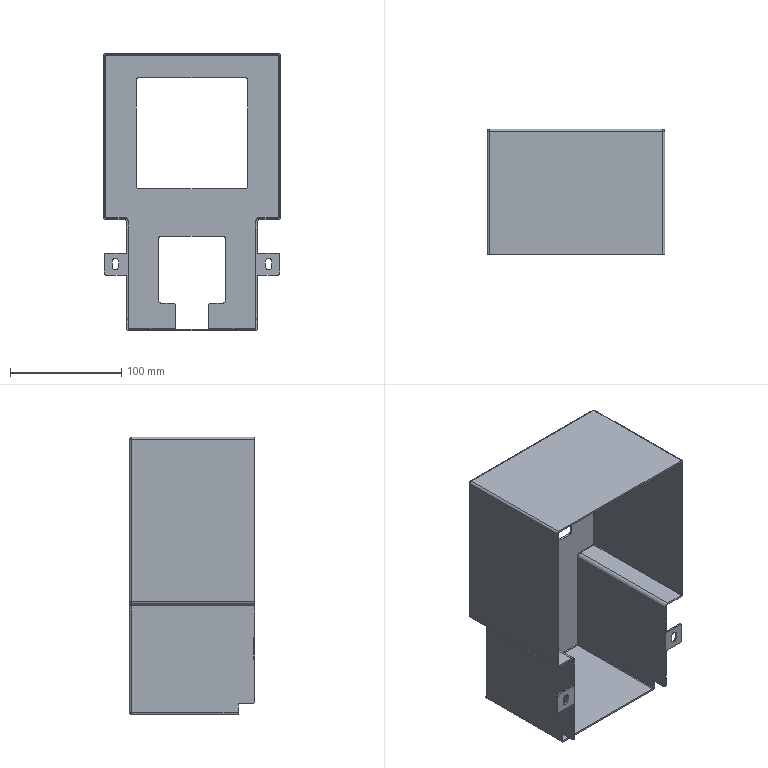Part | STEP file | ND25021-01-JDKM-10-BJ | 1 solid | 118 faces | box 160 x 113 x 250 mm | volume 164622 mm3 | cylinder 56 | plane 46 | sphere 12 | torus 4 | commonest cylinder face diameters 4 x33 1 x15 6 x6 7 x2